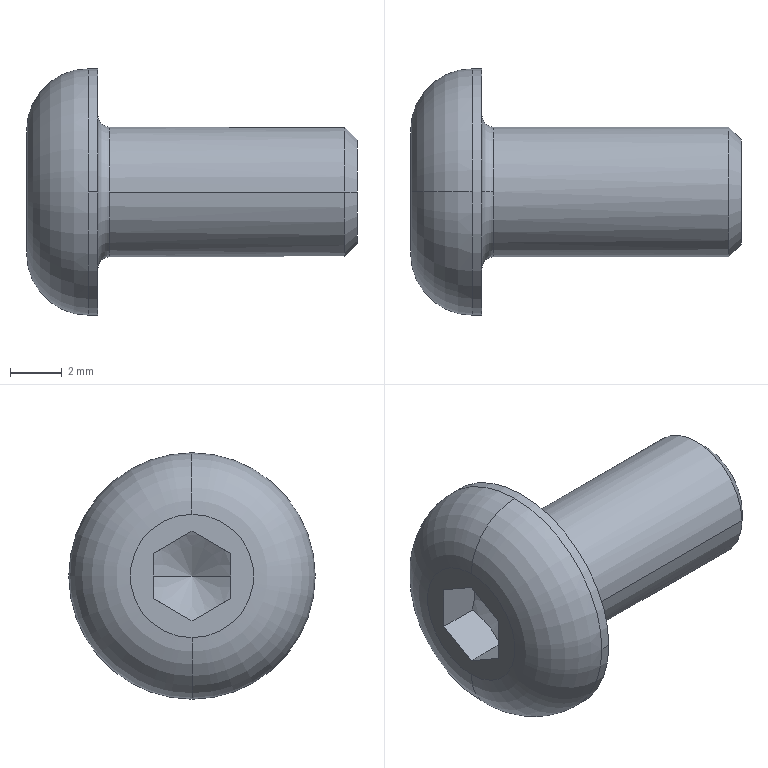Part | STEP file | ISO 7380-1 - M5 x 10 | 1 solid | 21 faces | box 12.75 x 9.5 x 9.5 mm | volume 343.038 mm3 | plane 9 | torus 4 | cylinder 4 | cone 4 | commonest cylinder face diameters 5 x2 9.5 x2